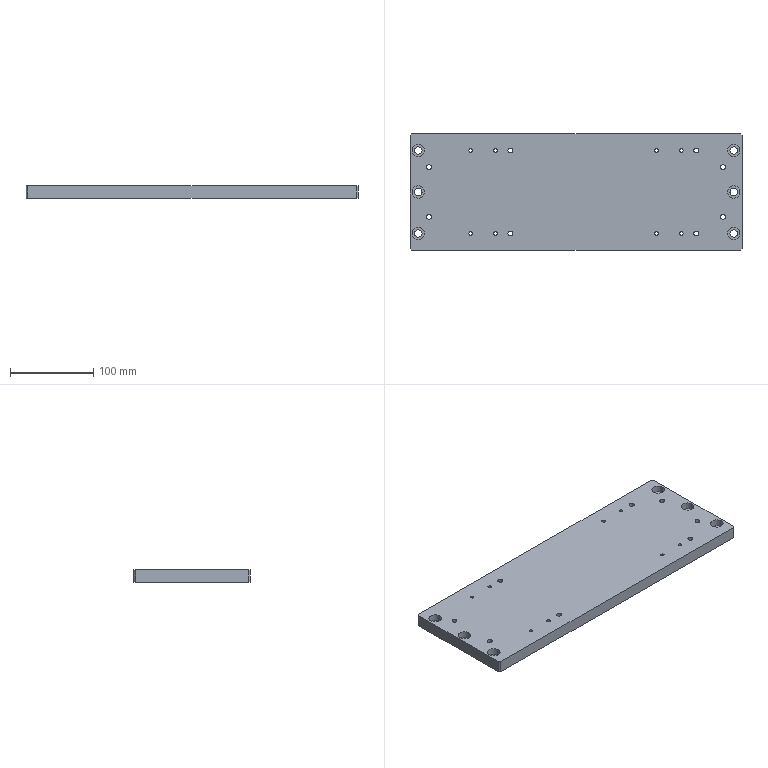Part | 1 solid | 52 faces | box 400 x 140 x 15 mm | volume 820295 mm3 | cylinder 32 | plane 16 | cone 4 | commonest cylinder face diameters 4.2 x8 6 x8 9 x6 15 x6 6.8 x4
STEP:
#1=CARTESIAN_POINT('',(-198.,70.,7.5));
#2=VERTEX_POINT('',#1);
#3=CARTESIAN_POINT('',(-200.,68.,7.5));
#4=VERTEX_POINT('',#3);
#5=CARTESIAN_POINT('',(-134.,134.,7.5));
#6=DIRECTION('',(-0.7071,-0.7071,0.));
#7=VECTOR('',#6,1000.);
#8=LINE('',#5,#7);
#9=EDGE_CURVE('',#2,#4,#8,.T.);
#10=ORIENTED_EDGE('',*,*,#9,.F.);
#11=CARTESIAN_POINT('',(-198.,70.,-7.5));
#12=VERTEX_POINT('',#11);
#13=CARTESIAN_POINT('',(-198.,70.,7.5));
#14=DIRECTION('',(0.,0.,1.));
#15=VECTOR('',#14,1000.);
#16=LINE('',#13,#15);
#17=EDGE_CURVE('',#12,#2,#16,.T.);
#18=ORIENTED_EDGE('',*,*,#17,.F.);
#19=CARTESIAN_POINT('',(-200.,68.,-7.5));
#20=VERTEX_POINT('',#19);
#21=CARTESIAN_POINT('',(-200.,68.,-7.5));
#22=DIRECTION('',(0.7071,0.7071,0.));
#23=VECTOR('',#22,1000.);
#24=LINE('',#21,#23);
#25=EDGE_CURVE('',#20,#12,#24,.T.);
#26=ORIENTED_EDGE('',*,*,#25,.F.);
#27=CARTESIAN_POINT('',(-200.,68.,7.5));
#28=DIRECTION('',(0.,0.,-1.));
#29=VECTOR('',#28,1000.);
#30=LINE('',#27,#29);
#31=EDGE_CURVE('',#4,#20,#30,.T.);
#32=ORIENTED_EDGE('',*,*,#31,.F.);
#33=EDGE_LOOP('',(#10,#18,#26,#32));
#34=FACE_BOUND('',#33,.T.);
#35=CARTESIAN_POINT('',(-200.,68.,7.5));
#36=DIRECTION('',(0.7071,-0.7071,0.));
#37=DIRECTION('',(0.,0.,-1.));
#38=AXIS2_PLACEMENT_3D('',#35,#36,#37);
#39=PLANE('',#38);
#40=ADVANCED_FACE('',(#34),#39,.F.);
#41=CARTESIAN_POINT('',(200.,68.,7.5));
#42=VERTEX_POINT('',#41);
#43=CARTESIAN_POINT('',(198.,70.,7.5));
#44=VERTEX_POINT('',#43);
#45=CARTESIAN_POINT('',(134.,134.,7.5));
#46=DIRECTION('',(-0.7071,0.7071,0.));
#47=VECTOR('',#46,1000.);
#48=LINE('',#45,#47);
#49=EDGE_CURVE('',#42,#44,#48,.T.);
#50=ORIENTED_EDGE('',*,*,#49,.F.);
#51=CARTESIAN_POINT('',(200.,68.,-7.5));
#52=VERTEX_POINT('',#51);
#53=CARTESIAN_POINT('',(200.,68.,7.5));
#54=DIRECTION('',(0.,0.,1.));
#55=VECTOR('',#54,1000.);
#56=LINE('',#53,#55);
#57=EDGE_CURVE('',#52,#42,#56,.T.);
#58=ORIENTED_EDGE('',*,*,#57,.F.);
#59=CARTESIAN_POINT('',(198.,70.,-7.5));
#60=VERTEX_POINT('',#59);
#61=CARTESIAN_POINT('',(198.,70.,-7.5));
#62=DIRECTION('',(0.7071,-0.7071,0.));
#63=VECTOR('',#62,1000.);
#64=LINE('',#61,#63);
#65=EDGE_CURVE('',#60,#52,#64,.T.);
#66=ORIENTED_EDGE('',*,*,#65,.F.);
#67=CARTESIAN_POINT('',(198.,70.,7.5));
#68=DIRECTION('',(0.,0.,-1.));
#69=VECTOR('',#68,1000.);
#70=LINE('',#67,#69);
#71=EDGE_CURVE('',#44,#60,#70,.T.);
#72=ORIENTED_EDGE('',*,*,#71,.F.);
#73=EDGE_LOOP('',(#50,#58,#66,#72));
#74=FACE_BOUND('',#73,.T.);
#75=CARTESIAN_POINT('',(198.,70.,7.5));
#76=DIRECTION('',(-0.7071,-0.7071,0.));
#77=DIRECTION('',(0.,0.,-1.));
#78=AXIS2_PLACEMENT_3D('',#75,#76,#77);
#79=PLANE('',#78);
#80=ADVANCED_FACE('',(#74),#79,.F.);
#81=CARTESIAN_POINT('',(-200.,-68.,7.5));
#82=VERTEX_POINT('',#81);
#83=CARTESIAN_POINT('',(-198.,-70.,7.5));
#84=VERTEX_POINT('',#83);
#85=CARTESIAN_POINT('',(-134.,-134.,7.5));
#86=DIRECTION('',(0.7071,-0.7071,0.));
#87=VECTOR('',#86,1000.);
#88=LINE('',#85,#87);
#89=EDGE_CURVE('',#82,#84,#88,.T.);
#90=ORIENTED_EDGE('',*,*,#89,.F.);
#91=CARTESIAN_POINT('',(-200.,-68.,-7.5));
#92=VERTEX_POINT('',#91);
#93=CARTESIAN_POINT('',(-200.,-68.,7.5));
#94=DIRECTION('',(0.,0.,1.));
#95=VECTOR('',#94,1000.);
#96=LINE('',#93,#95);
#97=EDGE_CURVE('',#92,#82,#96,.T.);
#98=ORIENTED_EDGE('',*,*,#97,.F.);
#99=CARTESIAN_POINT('',(-198.,-70.,-7.5));
#100=VERTEX_POINT('',#99);
#101=CARTESIAN_POINT('',(-198.,-70.,-7.5));
#102=DIRECTION('',(-0.7071,0.7071,0.));
#103=VECTOR('',#102,1000.);
#104=LINE('',#101,#103);
#105=EDGE_CURVE('',#100,#92,#104,.T.);
#106=ORIENTED_EDGE('',*,*,#105,.F.);
#107=CARTESIAN_POINT('',(-198.,-70.,7.5));
#108=DIRECTION('',(0.,0.,-1.));
#109=VECTOR('',#108,1000.);
#110=LINE('',#107,#109);
#111=EDGE_CURVE('',#84,#100,#110,.T.);
#112=ORIENTED_EDGE('',*,*,#111,.F.);
#113=EDGE_LOOP('',(#90,#98,#106,#112));
#114=FACE_BOUND('',#113,.T.);
#115=CARTESIAN_POINT('',(-198.,-70.,7.5));
#116=DIRECTION('',(0.7071,0.7071,0.));
#117=DIRECTION('',(0.,0.,-1.));
#118=AXIS2_PLACEMENT_3D('',#115,#116,#117);
#119=PLANE('',#118);
#120=ADVANCED_FACE('',(#114),#119,.F.);
#121=CARTESIAN_POINT('',(198.,-70.,7.5));
#122=VERTEX_POINT('',#121);
#123=CARTESIAN_POINT('',(200.,-68.,7.5));
#124=VERTEX_POINT('',#123);
#125=CARTESIAN_POINT('',(134.,-134.,7.5));
#126=DIRECTION('',(0.7071,0.7071,0.));
#127=VECTOR('',#126,1000.);
#128=LINE('',#125,#127);
#129=EDGE_CURVE('',#122,#124,#128,.T.);
#130=ORIENTED_EDGE('',*,*,#129,.F.);
#131=CARTESIAN_POINT('',(198.,-70.,-7.5));
#132=VERTEX_POINT('',#131);
#133=CARTESIAN_POINT('',(198.,-70.,7.5));
#134=DIRECTION('',(0.,0.,1.));
#135=VECTOR('',#134,1000.);
#136=LINE('',#133,#135);
#137=EDGE_CURVE('',#132,#122,#136,.T.);
#138=ORIENTED_EDGE('',*,*,#137,.F.);
#139=CARTESIAN_POINT('',(200.,-68.,-7.5));
#140=VERTEX_POINT('',#139);
#141=CARTESIAN_POINT('',(200.,-68.,-7.5));
#142=DIRECTION('',(-0.7071,-0.7071,0.));
#143=VECTOR('',#142,1000.);
#144=LINE('',#141,#143);
#145=EDGE_CURVE('',#140,#132,#144,.T.);
#146=ORIENTED_EDGE('',*,*,#145,.F.);
#147=CARTESIAN_POINT('',(200.,-68.,7.5));
#148=DIRECTION('',(0.,0.,-1.));
#149=VECTOR('',#148,1000.);
#150=LINE('',#147,#149);
#151=EDGE_CURVE('',#124,#140,#150,.T.);
#152=ORIENTED_EDGE('',*,*,#151,.F.);
#153=EDGE_LOOP('',(#130,#138,#146,#152));
#154=FACE_BOUND('',#153,.T.);
#155=CARTESIAN_POINT('',(200.,-68.,7.5));
#156=DIRECTION('',(-0.7071,0.7071,0.));
#157=DIRECTION('',(0.,0.,-1.));
#158=AXIS2_PLACEMENT_3D('',#155,#156,#157);
#159=PLANE('',#158);
#160=ADVANCED_FACE('',(#154),#159,.F.);
#161=CARTESIAN_POINT('',(-182.5,50.,-1.1));
#162=VERTEX_POINT('',#161);
#163=CARTESIAN_POINT('',(-190.,50.,-1.1));
#164=DIRECTION('',(0.,0.,1.));
#165=DIRECTION('',(1.,0.,0.));
#166=AXIS2_PLACEMENT_3D('',#163,#164,#165);
#167=CIRCLE('',#166,7.5);
#168=EDGE_CURVE('',#162,#162,#167,.T.);
#169=ORIENTED_EDGE('',*,*,#168,.T.);
#170=EDGE_LOOP('',(#169));
#171=FACE_BOUND('',#170,.T.);
#172=CARTESIAN_POINT('',(-185.5,50.,-1.1));
#173=VERTEX_POINT('',#172);
#174=CARTESIAN_POINT('',(-190.,50.,-1.1));
#175=DIRECTION('',(0.,0.,1.));
#176=DIRECTION('',(1.,0.,0.));
#177=AXIS2_PLACEMENT_3D('',#174,#175,#176);
#178=CIRCLE('',#177,4.5);
#179=EDGE_CURVE('',#173,#173,#178,.T.);
#180=ORIENTED_EDGE('',*,*,#179,.F.);
#181=EDGE_LOOP('',(#180));
#182=FACE_BOUND('',#181,.T.);
#183=CARTESIAN_POINT('',(-185.5,50.,-1.1));
#184=DIRECTION('',(0.,0.,-1.));
#185=DIRECTION('',(-1.,0.,0.));
#186=AXIS2_PLACEMENT_3D('',#183,#184,#185);
#187=PLANE('',#186);
#188=ADVANCED_FACE('',(#171,#182),#187,.F.);
#189=CARTESIAN_POINT('',(182.5,50.,-1.1));
#190=VERTEX_POINT('',#189);
#191=CARTESIAN_POINT('',(190.,50.,-1.1));
#192=DIRECTION('',(0.,0.,1.));
#193=DIRECTION('',(-1.,0.,0.));
#194=AXIS2_PLACEMENT_3D('',#191,#192,#193);
#195=CIRCLE('',#194,7.5);
#196=EDGE_CURVE('',#190,#190,#195,.T.);
#197=ORIENTED_EDGE('',*,*,#196,.T.);
#198=EDGE_LOOP('',(#197));
#199=FACE_BOUND('',#198,.T.);
#200=CARTESIAN_POINT('',(185.5,50.,-1.1));
#201=VERTEX_POINT('',#200);
#202=CARTESIAN_POINT('',(190.,50.,-1.1));
#203=DIRECTION('',(0.,0.,1.));
#204=DIRECTION('',(-1.,0.,0.));
#205=AXIS2_PLACEMENT_3D('',#202,#203,#204);
#206=CIRCLE('',#205,4.5);
#207=EDGE_CURVE('',#201,#201,#206,.T.);
#208=ORIENTED_EDGE('',*,*,#207,.F.);
#209=EDGE_LOOP('',(#208));
#210=FACE_BOUND('',#209,.T.);
#211=CARTESIAN_POINT('',(-185.5,50.,-1.1));
#212=DIRECTION('',(0.,0.,-1.));
#213=DIRECTION('',(-1.,0.,0.));
#214=AXIS2_PLACEMENT_3D('',#211,#212,#213);
#215=PLANE('',#214);
#216=ADVANCED_FACE('',(#199,#210),#215,.F.);
#217=CARTESIAN_POINT('',(-197.5,-50.,-1.1));
#218=VERTEX_POINT('',#217);
#219=CARTESIAN_POINT('',(-190.,-50.,-1.1));
#220=DIRECTION('',(0.,0.,1.));
#221=DIRECTION('',(-1.,0.,0.));
#222=AXIS2_PLACEMENT_3D('',#219,#220,#221);
#223=CIRCLE('',#222,7.5);
#224=EDGE_CURVE('',#218,#218,#223,.T.);
#225=ORIENTED_EDGE('',*,*,#224,.T.);
#226=EDGE_LOOP('',(#225));
#227=FACE_BOUND('',#226,.T.);
#228=CARTESIAN_POINT('',(-194.5,-50.,-1.1));
#229=VERTEX_POINT('',#228);
#230=CARTESIAN_POINT('',(-190.,-50.,-1.1));
#231=DIRECTION('',(0.,0.,1.));
#232=DIRECTION('',(-1.,0.,0.));
#233=AXIS2_PLACEMENT_3D('',#230,#231,#232);
#234=CIRCLE('',#233,4.5);
#235=EDGE_CURVE('',#229,#229,#234,.T.);
#236=ORIENTED_EDGE('',*,*,#235,.F.);
#237=EDGE_LOOP('',(#236));
#238=FACE_BOUND('',#237,.T.);
#239=CARTESIAN_POINT('',(-185.5,50.,-1.1));
#240=DIRECTION('',(0.,0.,-1.));
#241=DIRECTION('',(-1.,0.,0.));
#242=AXIS2_PLACEMENT_3D('',#239,#240,#241);
#243=PLANE('',#242);
#244=ADVANCED_FACE('',(#227,#238),#243,.F.);
#245=CARTESIAN_POINT('',(182.5,-50.,-1.1));
#246=VERTEX_POINT('',#245);
#247=CARTESIAN_POINT('',(190.,-50.,-1.1));
#248=DIRECTION('',(0.,0.,1.));
#249=DIRECTION('',(-1.,0.,0.));
#250=AXIS2_PLACEMENT_3D('',#247,#248,#249);
#251=CIRCLE('',#250,7.5);
#252=EDGE_CURVE('',#246,#246,#251,.T.);
#253=ORIENTED_EDGE('',*,*,#252,.T.);
#254=EDGE_LOOP('',(#253));
#255=FACE_BOUND('',#254,.T.);
#256=CARTESIAN_POINT('',(185.5,-50.,-1.1));
#257=VERTEX_POINT('',#256);
#258=CARTESIAN_POINT('',(190.,-50.,-1.1));
#259=DIRECTION('',(0.,0.,1.));
#260=DIRECTION('',(-1.,0.,0.));
#261=AXIS2_PLACEMENT_3D('',#258,#259,#260);
#262=CIRCLE('',#261,4.5);
#263=EDGE_CURVE('',#257,#257,#262,.T.);
#264=ORIENTED_EDGE('',*,*,#263,.F.);
#265=EDGE_LOOP('',(#264));
#266=FACE_BOUND('',#265,.T.);
#267=CARTESIAN_POINT('',(-185.5,50.,-1.1));
#268=DIRECTION('',(0.,0.,-1.));
#269=DIRECTION('',(-1.,0.,0.));
#270=AXIS2_PLACEMENT_3D('',#267,#268,#269);
#271=PLANE('',#270);
#272=ADVANCED_FACE('',(#255,#266),#271,.F.);
#273=CARTESIAN_POINT('',(182.5,0.,-1.1));
#274=VERTEX_POINT('',#273);
#275=CARTESIAN_POINT('',(190.,0.,-1.1));
#276=DIRECTION('',(0.,0.,1.));
#277=DIRECTION('',(-1.,0.,0.));
#278=AXIS2_PLACEMENT_3D('',#275,#276,#277);
#279=CIRCLE('',#278,7.5);
#280=EDGE_CURVE('',#274,#274,#279,.T.);
#281=ORIENTED_EDGE('',*,*,#280,.T.);
#282=EDGE_LOOP('',(#281));
#283=FACE_BOUND('',#282,.T.);
#284=CARTESIAN_POINT('',(185.5,0.,-1.1));
#285=VERTEX_POINT('',#284);
#286=CARTESIAN_POINT('',(190.,0.,-1.1));
#287=DIRECTION('',(0.,0.,1.));
#288=DIRECTION('',(-1.,0.,0.));
#289=AXIS2_PLACEMENT_3D('',#286,#287,#288);
#290=CIRCLE('',#289,4.5);
#291=EDGE_CURVE('',#285,#285,#290,.T.);
#292=ORIENTED_EDGE('',*,*,#291,.F.);
#293=EDGE_LOOP('',(#292));
#294=FACE_BOUND('',#293,.T.);
#295=CARTESIAN_POINT('',(-185.5,50.,-1.1));
#296=DIRECTION('',(0.,0.,-1.));
#297=DIRECTION('',(-1.,0.,0.));
#298=AXIS2_PLACEMENT_3D('',#295,#296,#297);
#299=PLANE('',#298);
#300=ADVANCED_FACE('',(#283,#294),#299,.F.);
#301=CARTESIAN_POINT('',(-197.5,0.,-1.1));
#302=VERTEX_POINT('',#301);
#303=CARTESIAN_POINT('',(-190.,0.,-1.1));
#304=DIRECTION('',(0.,0.,1.));
#305=DIRECTION('',(-1.,0.,0.));
#306=AXIS2_PLACEMENT_3D('',#303,#304,#305);
#307=CIRCLE('',#306,7.5);
#308=EDGE_CURVE('',#302,#302,#307,.T.);
#309=ORIENTED_EDGE('',*,*,#308,.T.);
#310=EDGE_LOOP('',(#309));
#311=FACE_BOUND('',#310,.T.);
#312=CARTESIAN_POINT('',(-194.5,0.,-1.1));
#313=VERTEX_POINT('',#312);
#314=CARTESIAN_POINT('',(-190.,0.,-1.1));
#315=DIRECTION('',(0.,0.,1.));
#316=DIRECTION('',(-1.,0.,0.));
#317=AXIS2_PLACEMENT_3D('',#314,#315,#316);
#318=CIRCLE('',#317,4.5);
#319=EDGE_CURVE('',#313,#313,#318,.T.);
#320=ORIENTED_EDGE('',*,*,#319,.F.);
#321=EDGE_LOOP('',(#320));
#322=FACE_BOUND('',#321,.T.);
#323=CARTESIAN_POINT('',(-185.5,50.,-1.1));
#324=DIRECTION('',(0.,0.,-1.));
#325=DIRECTION('',(-1.,0.,0.));
#326=AXIS2_PLACEMENT_3D('',#323,#324,#325);
#327=PLANE('',#326);
#328=ADVANCED_FACE('',(#311,#322),#327,.F.);
#329=CARTESIAN_POINT('',(200.,-70.,-7.5));
#330=DIRECTION('',(0.,1.,0.));
#331=VECTOR('',#330,1000.);
#332=LINE('',#329,#331);
#333=EDGE_CURVE('',#140,#52,#332,.T.);
#334=ORIENTED_EDGE('',*,*,#333,.F.);
#335=ORIENTED_EDGE('',*,*,#145,.T.);
#336=CARTESIAN_POINT('',(200.,-70.,-7.5));
#337=DIRECTION('',(1.,0.,0.));
#338=VECTOR('',#337,1000.);
#339=LINE('',#336,#338);
#340=EDGE_CURVE('',#100,#132,#339,.T.);
#341=ORIENTED_EDGE('',*,*,#340,.F.);
#342=ORIENTED_EDGE('',*,*,#105,.T.);
#343=CARTESIAN_POINT('',(-200.,-70.,-7.5));
#344=DIRECTION('',(0.,-1.,0.));
#345=VECTOR('',#344,1000.);
#346=LINE('',#343,#345);
#347=EDGE_CURVE('',#20,#92,#346,.T.);
#348=ORIENTED_EDGE('',*,*,#347,.F.);
#349=ORIENTED_EDGE('',*,*,#25,.T.);
#350=CARTESIAN_POINT('',(200.,70.,-7.5));
#351=DIRECTION('',(-1.,0.,0.));
#352=VECTOR('',#351,1000.);
#353=LINE('',#350,#352);
#354=EDGE_CURVE('',#60,#12,#353,.T.);
#355=ORIENTED_EDGE('',*,*,#354,.F.);
#356=ORIENTED_EDGE('',*,*,#65,.T.);
#357=EDGE_LOOP('',(#334,#335,#341,#342,#348,#349,#355,#356));
#358=FACE_BOUND('',#357,.T.);
#359=CARTESIAN_POINT('',(-124.9,-50.,-7.5));
#360=VERTEX_POINT('',#359);
#361=CARTESIAN_POINT('',(-127.,-50.,-7.5));
#362=DIRECTION('',(0.,0.,1.));
#363=DIRECTION('',(1.,0.,0.));
#364=AXIS2_PLACEMENT_3D('',#361,#362,#363);
#365=CIRCLE('',#364,2.1);
#366=EDGE_CURVE('',#360,#360,#365,.T.);
#367=ORIENTED_EDGE('',*,*,#366,.T.);
#368=EDGE_LOOP('',(#367));
#369=FACE_BOUND('',#368,.T.);
#370=CARTESIAN_POINT('',(-94.9,-50.,-7.5));
#371=VERTEX_POINT('',#370);
#372=CARTESIAN_POINT('',(-97.,-50.,-7.5));
#373=DIRECTION('',(0.,0.,1.));
#374=DIRECTION('',(1.,0.,0.));
#375=AXIS2_PLACEMENT_3D('',#372,#373,#374);
#376=CIRCLE('',#375,2.1);
#377=EDGE_CURVE('',#371,#371,#376,.T.);
#378=ORIENTED_EDGE('',*,*,#377,.T.);
#379=EDGE_LOOP('',(#378));
#380=FACE_BOUND('',#379,.T.);
#381=CARTESIAN_POINT('',(-94.9,50.,-7.5));
#382=VERTEX_POINT('',#381);
#383=CARTESIAN_POINT('',(-97.,50.,-7.5));
#384=DIRECTION('',(0.,0.,1.));
#385=DIRECTION('',(1.,0.,0.));
#386=AXIS2_PLACEMENT_3D('',#383,#384,#385);
#387=CIRCLE('',#386,2.1);
#388=EDGE_CURVE('',#382,#382,#387,.T.);
#389=ORIENTED_EDGE('',*,*,#388,.T.);
#390=EDGE_LOOP('',(#389));
#391=FACE_BOUND('',#390,.T.);
#392=CARTESIAN_POINT('',(-124.9,50.,-7.5));
#393=VERTEX_POINT('',#392);
#394=CARTESIAN_POINT('',(-127.,50.,-7.5));
#395=DIRECTION('',(0.,0.,1.));
#396=DIRECTION('',(1.,0.,0.));
#397=AXIS2_PLACEMENT_3D('',#394,#395,#396);
#398=CIRCLE('',#397,2.1);
#399=EDGE_CURVE('',#393,#393,#398,.T.);
#400=ORIENTED_EDGE('',*,*,#399,.T.);
#401=EDGE_LOOP('',(#400));
#402=FACE_BOUND('',#401,.T.);
#403=CARTESIAN_POINT('',(-76.,-50.,-7.5));
#404=VERTEX_POINT('',#403);
#405=CARTESIAN_POINT('',(-79.,-50.,-7.5));
#406=DIRECTION('',(0.,0.,1.));
#407=DIRECTION('',(1.,0.,0.));
#408=AXIS2_PLACEMENT_3D('',#405,#406,#407);
#409=CIRCLE('',#408,3.);
#410=EDGE_CURVE('',#404,#404,#409,.T.);
#411=ORIENTED_EDGE('',*,*,#410,.T.);
#412=EDGE_LOOP('',(#411));
#413=FACE_BOUND('',#412,.T.);
#414=CARTESIAN_POINT('',(-76.,50.,-7.5));
#415=VERTEX_POINT('',#414);
#416=CARTESIAN_POINT('',(-79.,50.,-7.5));
#417=DIRECTION('',(0.,0.,1.));
#418=DIRECTION('',(1.,0.,0.));
#419=AXIS2_PLACEMENT_3D('',#416,#417,#418);
#420=CIRCLE('',#419,3.);
#421=EDGE_CURVE('',#415,#415,#420,.T.);
#422=ORIENTED_EDGE('',*,*,#421,.T.);
#423=EDGE_LOOP('',(#422));
#424=FACE_BOUND('',#423,.T.);
#425=CARTESIAN_POINT('',(99.1,50.,-7.5));
#426=VERTEX_POINT('',#425);
#427=CARTESIAN_POINT('',(97.,50.,-7.5));
#428=DIRECTION('',(0.,0.,1.));
#429=DIRECTION('',(1.,0.,0.));
#430=AXIS2_PLACEMENT_3D('',#427,#428,#429);
#431=CIRCLE('',#430,2.1);
#432=EDGE_CURVE('',#426,#426,#431,.T.);
#433=ORIENTED_EDGE('',*,*,#432,.T.);
#434=EDGE_LOOP('',(#433));
#435=FACE_BOUND('',#434,.T.);
#436=CARTESIAN_POINT('',(99.1,-50.,-7.5));
#437=VERTEX_POINT('',#436);
#438=CARTESIAN_POINT('',(97.,-50.,-7.5));
#439=DIRECTION('',(0.,0.,1.));
#440=DIRECTION('',(1.,0.,0.));
#441=AXIS2_PLACEMENT_3D('',#438,#439,#440);
#442=CIRCLE('',#441,2.1);
#443=EDGE_CURVE('',#437,#437,#442,.T.);
#444=ORIENTED_EDGE('',*,*,#443,.T.);
#445=EDGE_LOOP('',(#444));
#446=FACE_BOUND('',#445,.T.);
#447=CARTESIAN_POINT('',(129.1,-50.,-7.5));
#448=VERTEX_POINT('',#447);
#449=CARTESIAN_POINT('',(127.,-50.,-7.5));
#450=DIRECTION('',(0.,0.,1.));
#451=DIRECTION('',(1.,0.,0.));
#452=AXIS2_PLACEMENT_3D('',#449,#450,#451);
#453=CIRCLE('',#452,2.1);
#454=EDGE_CURVE('',#448,#448,#453,.T.);
#455=ORIENTED_EDGE('',*,*,#454,.T.);
#456=EDGE_LOOP('',(#455));
#457=FACE_BOUND('',#456,.T.);
#458=CARTESIAN_POINT('',(129.1,50.,-7.5));
#459=VERTEX_POINT('',#458);
#460=CARTESIAN_POINT('',(127.,50.,-7.5));
#461=DIRECTION('',(0.,0.,1.));
#462=DIRECTION('',(1.,0.,0.));
#463=AXIS2_PLACEMENT_3D('',#460,#461,#462);
#464=CIRCLE('',#463,2.1);
#465=EDGE_CURVE('',#459,#459,#464,.T.);
#466=ORIENTED_EDGE('',*,*,#465,.T.);
#467=EDGE_LOOP('',(#466));
#468=FACE_BOUND('',#467,.T.);
#469=CARTESIAN_POINT('',(148.,-50.,-7.5));
#470=VERTEX_POINT('',#469);
#471=CARTESIAN_POINT('',(145.,-50.,-7.5));
#472=DIRECTION('',(0.,0.,1.));
#473=DIRECTION('',(1.,0.,0.));
#474=AXIS2_PLACEMENT_3D('',#471,#472,#473);
#475=CIRCLE('',#474,3.);
#476=EDGE_CURVE('',#470,#470,#475,.T.);
#477=ORIENTED_EDGE('',*,*,#476,.T.);
#478=EDGE_LOOP('',(#477));
#479=FACE_BOUND('',#478,.T.);
#480=CARTESIAN_POINT('',(148.,50.,-7.5));
#481=VERTEX_POINT('',#480);
#482=CARTESIAN_POINT('',(145.,50.,-7.5));
#483=DIRECTION('',(0.,0.,1.));
#484=DIRECTION('',(1.,0.,0.));
#485=AXIS2_PLACEMENT_3D('',#482,#483,#484);
#486=CIRCLE('',#485,3.);
#487=EDGE_CURVE('',#481,#481,#486,.T.);
#488=ORIENTED_EDGE('',*,*,#487,.T.);
#489=EDGE_LOOP('',(#488));
#490=FACE_BOUND('',#489,.T.);
#491=CARTESIAN_POINT('',(-185.5,0.,-7.5));
#492=VERTEX_POINT('',#491);
#493=CARTESIAN_POINT('',(-190.,0.,-7.5));
#494=DIRECTION('',(0.,0.,1.));
#495=DIRECTION('',(1.,0.,0.));
#496=AXIS2_PLACEMENT_3D('',#493,#494,#495);
#497=CIRCLE('',#496,4.5);
#498=EDGE_CURVE('',#492,#492,#497,.T.);
#499=ORIENTED_EDGE('',*,*,#498,.T.);
#500=EDGE_LOOP('',(#499));
#501=FACE_BOUND('',#500,.T.);
#502=CARTESIAN_POINT('',(194.5,0.,-7.5));
#503=VERTEX_POINT('',#502);
#504=CARTESIAN_POINT('',(190.,0.,-7.5));
#505=DIRECTION('',(0.,0.,1.));
#506=DIRECTION('',(1.,0.,0.));
#507=AXIS2_PLACEMENT_3D('',#504,#505,#506);
#508=CIRCLE('',#507,4.5);
#509=EDGE_CURVE('',#503,#503,#508,.T.);
#510=ORIENTED_EDGE('',*,*,#509,.T.);
#511=EDGE_LOOP('',(#510));
#512=FACE_BOUND('',#511,.T.);
#513=CARTESIAN_POINT('',(194.5,-50.,-7.5));
#514=VERTEX_POINT('',#513);
#515=CARTESIAN_POINT('',(190.,-50.,-7.5));
#516=DIRECTION('',(0.,0.,1.));
#517=DIRECTION('',(1.,0.,0.));
#518=AXIS2_PLACEMENT_3D('',#515,#516,#517);
#519=CIRCLE('',#518,4.5);
#520=EDGE_CURVE('',#514,#514,#519,.T.);
#521=ORIENTED_EDGE('',*,*,#520,.T.);
#522=EDGE_LOOP('',(#521));
#523=FACE_BOUND('',#522,.T.);
#524=CARTESIAN_POINT('',(-185.5,-50.,-7.5));
#525=VERTEX_POINT('',#524);
#526=CARTESIAN_POINT('',(-190.,-50.,-7.5));
#527=DIRECTION('',(0.,0.,1.));
#528=DIRECTION('',(1.,0.,0.));
#529=AXIS2_PLACEMENT_3D('',#526,#527,#528);
#530=CIRCLE('',#529,4.5);
#531=EDGE_CURVE('',#525,#525,#530,.T.);
#532=ORIENTED_EDGE('',*,*,#531,.T.);
#533=EDGE_LOOP('',(#532));
#534=FACE_BOUND('',#533,.T.);
#535=CARTESIAN_POINT('',(194.5,50.,-7.5));
#536=VERTEX_POINT('',#535);
#537=CARTESIAN_POINT('',(190.,50.,-7.5));
#538=DIRECTION('',(0.,0.,1.));
#539=DIRECTION('',(1.,0.,0.));
#540=AXIS2_PLACEMENT_3D('',#537,#538,#539);
#541=CIRCLE('',#540,4.5);
#542=EDGE_CURVE('',#536,#536,#541,.T.);
#543=ORIENTED_EDGE('',*,*,#542,.T.);
#544=EDGE_LOOP('',(#543));
#545=FACE_BOUND('',#544,.T.);
#546=CARTESIAN_POINT('',(-185.5,50.,-7.5));
#547=VERTEX_POINT('',#546);
#548=CARTESIAN_POINT('',(-190.,50.,-7.5));
#549=DIRECTION('',(0.,0.,1.));
#550=DIRECTION('',(1.,0.,0.));
#551=AXIS2_PLACEMENT_3D('',#548,#549,#550);
#552=CIRCLE('',#551,4.5);
#553=EDGE_CURVE('',#547,#547,#552,.T.);
#554=ORIENTED_EDGE('',*,*,#553,.T.);
#555=EDGE_LOOP('',(#554));
#556=FACE_BOUND('',#555,.T.);
#557=CARTESIAN_POINT('',(-174.,-30.,-7.5));
#558=VERTEX_POINT('',#557);
#559=CARTESIAN_POINT('',(-177.,-30.,-7.5));
#560=DIRECTION('',(0.,0.,1.));
#561=DIRECTION('',(1.,0.,0.));
#562=AXIS2_PLACEMENT_3D('',#559,#560,#561);
#563=CIRCLE('',#562,3.);
#564=EDGE_CURVE('',#558,#558,#563,.T.);
#565=ORIENTED_EDGE('',*,*,#564,.T.);
#566=EDGE_LOOP('',(#565));
#567=FACE_BOUND('',#566,.T.);
#568=CARTESIAN_POINT('',(-174.,30.,-7.5));
#569=VERTEX_POINT('',#568);
#570=CARTESIAN_POINT('',(-177.,30.,-7.5));
#571=DIRECTION('',(0.,0.,1.));
#572=DIRECTION('',(1.,0.,0.));
#573=AXIS2_PLACEMENT_3D('',#570,#571,#572);
#574=CIRCLE('',#573,3.);
#575=EDGE_CURVE('',#569,#569,#574,.T.);
#576=ORIENTED_EDGE('',*,*,#575,.T.);
#577=EDGE_LOOP('',(#576));
#578=FACE_BOUND('',#577,.T.);
#579=CARTESIAN_POINT('',(180.,-30.,-7.5));
#580=VERTEX_POINT('',#579);
#581=CARTESIAN_POINT('',(177.,-30.,-7.5));
#582=DIRECTION('',(0.,0.,1.));
#583=DIRECTION('',(1.,0.,0.));
#584=AXIS2_PLACEMENT_3D('',#581,#582,#583);
#585=CIRCLE('',#584,3.);
#586=EDGE_CURVE('',#580,#580,#585,.T.);
#587=ORIENTED_EDGE('',*,*,#586,.T.);
#588=EDGE_LOOP('',(#587));
#589=FACE_BOUND('',#588,.T.);
#590=CARTESIAN_POINT('',(180.,30.,-7.5));
#591=VERTEX_POINT('',#590);
#592=CARTESIAN_POINT('',(177.,30.,-7.5));
#593=DIRECTION('',(0.,0.,1.));
#594=DIRECTION('',(1.,0.,0.));
#595=AXIS2_PLACEMENT_3D('',#592,#593,#594);
#596=CIRCLE('',#595,3.);
#597=EDGE_CURVE('',#591,#591,#596,.T.);
#598=ORIENTED_EDGE('',*,*,#597,.T.);
#599=EDGE_LOOP('',(#598));
#600=FACE_BOUND('',#599,.T.);
#601=CARTESIAN_POINT('',(0.,0.,-7.5));
#602=DIRECTION('',(0.,0.,1.));
#603=DIRECTION('',(1.,0.,0.));
#604=AXIS2_PLACEMENT_3D('',#601,#602,#603);
#605=PLANE('',#604);
#606=ADVANCED_FACE('',(#358,#369,#380,#391,#402,#413,#424,#435,#446,#457,#468,#479,#490,#501,#512,#523,#534,#545,#556,#567,#578,#589,#600),#605,.F.);
#607=CARTESIAN_POINT('',(200.,-70.,7.5));
#608=DIRECTION('',(1.,0.,0.));
#609=VECTOR('',#608,1000.);
#610=LINE('',#607,#609);
#611=EDGE_CURVE('',#84,#122,#610,.T.);
#612=ORIENTED_EDGE('',*,*,#611,.T.);
#613=ORIENTED_EDGE('',*,*,#129,.T.);
#614=CARTESIAN_POINT('',(200.,-70.,7.5));
#615=DIRECTION('',(0.,1.,0.));
#616=VECTOR('',#615,1000.);
#617=LINE('',#614,#616);
#618=EDGE_CURVE('',#124,#42,#617,.T.);
#619=ORIENTED_EDGE('',*,*,#618,.T.);
#620=ORIENTED_EDGE('',*,*,#49,.T.);
#621=CARTESIAN_POINT('',(200.,70.,7.5));
#622=DIRECTION('',(-1.,0.,0.));
#623=VECTOR('',#622,1000.);
#624=LINE('',#621,#623);
#625=EDGE_CURVE('',#44,#2,#624,.T.);
#626=ORIENTED_EDGE('',*,*,#625,.T.);
#627=ORIENTED_EDGE('',*,*,#9,.T.);
#628=CARTESIAN_POINT('',(-200.,-70.,7.5));
#629=DIRECTION('',(0.,-1.,0.));
#630=VECTOR('',#629,1000.);
#631=LINE('',#628,#630);
#632=EDGE_CURVE('',#4,#82,#631,.T.);
#633=ORIENTED_EDGE('',*,*,#632,.T.);
#634=ORIENTED_EDGE('',*,*,#89,.T.);
#635=EDGE_LOOP('',(#612,#613,#619,#620,#626,#627,#633,#634));
#636=FACE_BOUND('',#635,.T.);
#637=CARTESIAN_POINT('',(-124.9,-50.,7.5));
#638=VERTEX_POINT('',#637);
#639=CARTESIAN_POINT('',(-127.,-50.,7.5));
#640=DIRECTION('',(0.,0.,1.));
#641=DIRECTION('',(1.,0.,0.));
#642=AXIS2_PLACEMENT_3D('',#639,#640,#641);
#643=CIRCLE('',#642,2.1);
#644=EDGE_CURVE('',#638,#638,#643,.T.);
#645=ORIENTED_EDGE('',*,*,#644,.F.);
#646=EDGE_LOOP('',(#645));
#647=FACE_BOUND('',#646,.T.);
#648=CARTESIAN_POINT('',(-94.9,-50.,7.5));
#649=VERTEX_POINT('',#648);
#650=CARTESIAN_POINT('',(-97.,-50.,7.5));
#651=DIRECTION('',(0.,0.,1.));
#652=DIRECTION('',(1.,0.,0.));
#653=AXIS2_PLACEMENT_3D('',#650,#651,#652);
#654=CIRCLE('',#653,2.1);
#655=EDGE_CURVE('',#649,#649,#654,.T.);
#656=ORIENTED_EDGE('',*,*,#655,.F.);
#657=EDGE_LOOP('',(#656));
#658=FACE_BOUND('',#657,.T.);
#659=CARTESIAN_POINT('',(-94.9,50.,7.5));
#660=VERTEX_POINT('',#659);
#661=CARTESIAN_POINT('',(-97.,50.,7.5));
#662=DIRECTION('',(0.,0.,1.));
#663=DIRECTION('',(1.,0.,0.));
#664=AXIS2_PLACEMENT_3D('',#661,#662,#663);
#665=CIRCLE('',#664,2.1);
#666=EDGE_CURVE('',#660,#660,#665,.T.);
#667=ORIENTED_EDGE('',*,*,#666,.F.);
#668=EDGE_LOOP('',(#667));
#669=FACE_BOUND('',#668,.T.);
#670=CARTESIAN_POINT('',(-124.9,50.,7.5));
#671=VERTEX_POINT('',#670);
#672=CARTESIAN_POINT('',(-127.,50.,7.5));
#673=DIRECTION('',(0.,0.,1.));
#674=DIRECTION('',(1.,0.,0.));
#675=AXIS2_PLACEMENT_3D('',#672,#673,#674);
#676=CIRCLE('',#675,2.1);
#677=EDGE_CURVE('',#671,#671,#676,.T.);
#678=ORIENTED_EDGE('',*,*,#677,.F.);
#679=EDGE_LOOP('',(#678));
#680=FACE_BOUND('',#679,.T.);
#681=CARTESIAN_POINT('',(-76.,-50.,7.5));
#682=VERTEX_POINT('',#681);
#683=CARTESIAN_POINT('',(-79.,-50.,7.5));
#684=DIRECTION('',(0.,0.,1.));
#685=DIRECTION('',(1.,0.,0.));
#686=AXIS2_PLACEMENT_3D('',#683,#684,#685);
#687=CIRCLE('',#686,3.);
#688=EDGE_CURVE('',#682,#682,#687,.T.);
#689=ORIENTED_EDGE('',*,*,#688,.F.);
#690=EDGE_LOOP('',(#689));
#691=FACE_BOUND('',#690,.T.);
#692=CARTESIAN_POINT('',(-76.,50.,7.5));
#693=VERTEX_POINT('',#692);
#694=CARTESIAN_POINT('',(-79.,50.,7.5));
#695=DIRECTION('',(0.,0.,1.));
#696=DIRECTION('',(1.,0.,0.));
#697=AXIS2_PLACEMENT_3D('',#694,#695,#696);
#698=CIRCLE('',#697,3.);
#699=EDGE_CURVE('',#693,#693,#698,.T.);
#700=ORIENTED_EDGE('',*,*,#699,.F.);
#701=EDGE_LOOP('',(#700));
#702=FACE_BOUND('',#701,.T.);
#703=CARTESIAN_POINT('',(99.1,50.,7.5));
#704=VERTEX_POINT('',#703);
#705=CARTESIAN_POINT('',(97.,50.,7.5));
#706=DIRECTION('',(0.,0.,1.));
#707=DIRECTION('',(1.,0.,0.));
#708=AXIS2_PLACEMENT_3D('',#705,#706,#707);
#709=CIRCLE('',#708,2.1);
#710=EDGE_CURVE('',#704,#704,#709,.T.);
#711=ORIENTED_EDGE('',*,*,#710,.F.);
#712=EDGE_LOOP('',(#711));
#713=FACE_BOUND('',#712,.T.);
#714=CARTESIAN_POINT('',(99.1,-50.,7.5));
#715=VERTEX_POINT('',#714);
#716=CARTESIAN_POINT('',(97.,-50.,7.5));
#717=DIRECTION('',(0.,0.,1.));
#718=DIRECTION('',(1.,0.,0.));
#719=AXIS2_PLACEMENT_3D('',#716,#717,#718);
#720=CIRCLE('',#719,2.1);
#721=EDGE_CURVE('',#715,#715,#720,.T.);
#722=ORIENTED_EDGE('',*,*,#721,.F.);
#723=EDGE_LOOP('',(#722));
#724=FACE_BOUND('',#723,.T.);
#725=CARTESIAN_POINT('',(129.1,-50.,7.5));
#726=VERTEX_POINT('',#725);
#727=CARTESIAN_POINT('',(127.,-50.,7.5));
#728=DIRECTION('',(0.,0.,1.));
#729=DIRECTION('',(1.,0.,0.));
#730=AXIS2_PLACEMENT_3D('',#727,#728,#729);
#731=CIRCLE('',#730,2.1);
#732=EDGE_CURVE('',#726,#726,#731,.T.);
#733=ORIENTED_EDGE('',*,*,#732,.F.);
#734=EDGE_LOOP('',(#733));
#735=FACE_BOUND('',#734,.T.);
#736=CARTESIAN_POINT('',(129.1,50.,7.5));
#737=VERTEX_POINT('',#736);
#738=CARTESIAN_POINT('',(127.,50.,7.5));
#739=DIRECTION('',(0.,0.,1.));
#740=DIRECTION('',(1.,0.,0.));
#741=AXIS2_PLACEMENT_3D('',#738,#739,#740);
#742=CIRCLE('',#741,2.1);
#743=EDGE_CURVE('',#737,#737,#742,.T.);
#744=ORIENTED_EDGE('',*,*,#743,.F.);
#745=EDGE_LOOP('',(#744));
#746=FACE_BOUND('',#745,.T.);
#747=CARTESIAN_POINT('',(148.,-50.,7.5));
#748=VERTEX_POINT('',#747);
#749=CARTESIAN_POINT('',(145.,-50.,7.5));
#750=DIRECTION('',(0.,0.,1.));
#751=DIRECTION('',(1.,0.,0.));
#752=AXIS2_PLACEMENT_3D('',#749,#750,#751);
#753=CIRCLE('',#752,3.);
#754=EDGE_CURVE('',#748,#748,#753,.T.);
#755=ORIENTED_EDGE('',*,*,#754,.F.);
#756=EDGE_LOOP('',(#755));
#757=FACE_BOUND('',#756,.T.);
#758=CARTESIAN_POINT('',(148.,50.,7.5));
#759=VERTEX_POINT('',#758);
#760=CARTESIAN_POINT('',(145.,50.,7.5));
#761=DIRECTION('',(0.,0.,1.));
#762=DIRECTION('',(1.,0.,0.));
#763=AXIS2_PLACEMENT_3D('',#760,#761,#762);
#764=CIRCLE('',#763,3.);
#765=EDGE_CURVE('',#759,#759,#764,.T.);
#766=ORIENTED_EDGE('',*,*,#765,.F.);
#767=EDGE_LOOP('',(#766));
#768=FACE_BOUND('',#767,.T.);
#769=CARTESIAN_POINT('',(-182.5,0.,7.5));
#770=VERTEX_POINT('',#769);
#771=CARTESIAN_POINT('',(-190.,0.,7.5));
#772=DIRECTION('',(0.,0.,1.));
#773=DIRECTION('',(1.,0.,0.));
#774=AXIS2_PLACEMENT_3D('',#771,#772,#773);
#775=CIRCLE('',#774,7.5);
#776=EDGE_CURVE('',#770,#770,#775,.T.);
#777=ORIENTED_EDGE('',*,*,#776,.F.);
#778=EDGE_LOOP('',(#777));
#779=FACE_BOUND('',#778,.T.);
#780=CARTESIAN_POINT('',(197.5,0.,7.5));
#781=VERTEX_POINT('',#780);
#782=CARTESIAN_POINT('',(190.,0.,7.5));
#783=DIRECTION('',(0.,0.,1.));
#784=DIRECTION('',(1.,0.,0.));
#785=AXIS2_PLACEMENT_3D('',#782,#783,#784);
#786=CIRCLE('',#785,7.5);
#787=EDGE_CURVE('',#781,#781,#786,.T.);
#788=ORIENTED_EDGE('',*,*,#787,.F.);
#789=EDGE_LOOP('',(#788));
#790=FACE_BOUND('',#789,.T.);
#791=CARTESIAN_POINT('',(197.5,-50.,7.5));
#792=VERTEX_POINT('',#791);
#793=CARTESIAN_POINT('',(190.,-50.,7.5));
#794=DIRECTION('',(0.,0.,1.));
#795=DIRECTION('',(1.,0.,0.));
#796=AXIS2_PLACEMENT_3D('',#793,#794,#795);
#797=CIRCLE('',#796,7.5);
#798=EDGE_CURVE('',#792,#792,#797,.T.);
#799=ORIENTED_EDGE('',*,*,#798,.F.);
#800=EDGE_LOOP('',(#799));
#801=FACE_BOUND('',#800,.T.);
#802=CARTESIAN_POINT('',(-182.5,-50.,7.5));
#803=VERTEX_POINT('',#802);
#804=CARTESIAN_POINT('',(-190.,-50.,7.5));
#805=DIRECTION('',(0.,0.,1.));
#806=DIRECTION('',(1.,0.,0.));
#807=AXIS2_PLACEMENT_3D('',#804,#805,#806);
#808=CIRCLE('',#807,7.5);
#809=EDGE_CURVE('',#803,#803,#808,.T.);
#810=ORIENTED_EDGE('',*,*,#809,.F.);
#811=EDGE_LOOP('',(#810));
#812=FACE_BOUND('',#811,.T.);
#813=CARTESIAN_POINT('',(197.5,50.,7.5));
#814=VERTEX_POINT('',#813);
#815=CARTESIAN_POINT('',(190.,50.,7.5));
#816=DIRECTION('',(0.,0.,1.));
#817=DIRECTION('',(1.,0.,0.));
#818=AXIS2_PLACEMENT_3D('',#815,#816,#817);
#819=CIRCLE('',#818,7.5);
#820=EDGE_CURVE('',#814,#814,#819,.T.);
#821=ORIENTED_EDGE('',*,*,#820,.F.);
#822=EDGE_LOOP('',(#821));
#823=FACE_BOUND('',#822,.T.);
#824=CARTESIAN_POINT('',(-182.5,50.,7.5));
#825=VERTEX_POINT('',#824);
#826=CARTESIAN_POINT('',(-190.,50.,7.5));
#827=DIRECTION('',(0.,0.,1.));
#828=DIRECTION('',(1.,0.,0.));
#829=AXIS2_PLACEMENT_3D('',#826,#827,#828);
#830=CIRCLE('',#829,7.5);
#831=EDGE_CURVE('',#825,#825,#830,.T.);
#832=ORIENTED_EDGE('',*,*,#831,.F.);
#833=EDGE_LOOP('',(#832));
#834=FACE_BOUND('',#833,.T.);
#835=CARTESIAN_POINT('',(-174.,-30.,7.5));
#836=VERTEX_POINT('',#835);
#837=CARTESIAN_POINT('',(-177.,-30.,7.5));
#838=DIRECTION('',(0.,0.,1.));
#839=DIRECTION('',(1.,0.,0.));
#840=AXIS2_PLACEMENT_3D('',#837,#838,#839);
#841=CIRCLE('',#840,3.);
#842=EDGE_CURVE('',#836,#836,#841,.T.);
#843=ORIENTED_EDGE('',*,*,#842,.F.);
#844=EDGE_LOOP('',(#843));
#845=FACE_BOUND('',#844,.T.);
#846=CARTESIAN_POINT('',(-174.,30.,7.5));
#847=VERTEX_POINT('',#846);
#848=CARTESIAN_POINT('',(-177.,30.,7.5));
#849=DIRECTION('',(0.,0.,1.));
#850=DIRECTION('',(1.,0.,0.));
#851=AXIS2_PLACEMENT_3D('',#848,#849,#850);
#852=CIRCLE('',#851,3.);
#853=EDGE_CURVE('',#847,#847,#852,.T.);
#854=ORIENTED_EDGE('',*,*,#853,.F.);
#855=EDGE_LOOP('',(#854));
#856=FACE_BOUND('',#855,.T.);
#857=CARTESIAN_POINT('',(180.,-30.,7.5));
#858=VERTEX_POINT('',#857);
#859=CARTESIAN_POINT('',(177.,-30.,7.5));
#860=DIRECTION('',(0.,0.,1.));
#861=DIRECTION('',(1.,0.,0.));
#862=AXIS2_PLACEMENT_3D('',#859,#860,#861);
#863=CIRCLE('',#862,3.);
#864=EDGE_CURVE('',#858,#858,#863,.T.);
#865=ORIENTED_EDGE('',*,*,#864,.F.);
#866=EDGE_LOOP('',(#865));
#867=FACE_BOUND('',#866,.T.);
#868=CARTESIAN_POINT('',(180.,30.,7.5));
#869=VERTEX_POINT('',#868);
#870=CARTESIAN_POINT('',(177.,30.,7.5));
#871=DIRECTION('',(0.,0.,1.));
#872=DIRECTION('',(1.,0.,0.));
#873=AXIS2_PLACEMENT_3D('',#870,#871,#872);
#874=CIRCLE('',#873,3.);
#875=EDGE_CURVE('',#869,#869,#874,.T.);
#876=ORIENTED_EDGE('',*,*,#875,.F.);
#877=EDGE_LOOP('',(#876));
#878=FACE_BOUND('',#877,.T.);
#879=CARTESIAN_POINT('',(0.,0.,7.5));
#880=DIRECTION('',(0.,0.,1.));
#881=DIRECTION('',(1.,0.,0.));
#882=AXIS2_PLACEMENT_3D('',#879,#880,#881);
#883=PLANE('',#882);
#884=ADVANCED_FACE('',(#636,#647,#658,#669,#680,#691,#702,#713,#724,#735,#746,#757,#768,#779,#790,#801,#812,#823,#834,#845,#856,#867,#878),#883,.T.);
#885=ORIENTED_EDGE('',*,*,#625,.F.);
#886=ORIENTED_EDGE('',*,*,#71,.T.);
#887=ORIENTED_EDGE('',*,*,#354,.T.);
#888=ORIENTED_EDGE('',*,*,#17,.T.);
#889=EDGE_LOOP('',(#885,#886,#887,#888));
#890=FACE_BOUND('',#889,.T.);
#891=CARTESIAN_POINT('',(-165.,70.,3.4));
#892=VERTEX_POINT('',#891);
#893=CARTESIAN_POINT('',(-165.,70.,0.));
#894=DIRECTION('',(0.,1.,0.));
#895=DIRECTION('',(0.,0.,1.));
#896=AXIS2_PLACEMENT_3D('',#893,#894,#895);
#897=CIRCLE('',#896,3.4);
#898=EDGE_CURVE('',#892,#892,#897,.T.);
#899=ORIENTED_EDGE('',*,*,#898,.F.);
#900=EDGE_LOOP('',(#899));
#901=FACE_BOUND('',#900,.T.);
#902=CARTESIAN_POINT('',(-55.,70.,3.4));
#903=VERTEX_POINT('',#902);
#904=CARTESIAN_POINT('',(-55.,70.,0.));
#905=DIRECTION('',(0.,1.,0.));
#906=DIRECTION('',(0.,0.,1.));
#907=AXIS2_PLACEMENT_3D('',#904,#905,#906);
#908=CIRCLE('',#907,3.4);
#909=EDGE_CURVE('',#903,#903,#908,.T.);
#910=ORIENTED_EDGE('',*,*,#909,.F.);
#911=EDGE_LOOP('',(#910));
#912=FACE_BOUND('',#911,.T.);
#913=CARTESIAN_POINT('',(55.,70.,3.4));
#914=VERTEX_POINT('',#913);
#915=CARTESIAN_POINT('',(55.,70.,0.));
#916=DIRECTION('',(0.,1.,0.));
#917=DIRECTION('',(0.,0.,1.));
#918=AXIS2_PLACEMENT_3D('',#915,#916,#917);
#919=CIRCLE('',#918,3.4);
#920=EDGE_CURVE('',#914,#914,#919,.T.);
#921=ORIENTED_EDGE('',*,*,#920,.F.);
#922=EDGE_LOOP('',(#921));
#923=FACE_BOUND('',#922,.T.);
#924=CARTESIAN_POINT('',(165.,70.,3.4));
#925=VERTEX_POINT('',#924);
#926=CARTESIAN_POINT('',(165.,70.,0.));
#927=DIRECTION('',(0.,1.,0.));
#928=DIRECTION('',(0.,0.,1.));
#929=AXIS2_PLACEMENT_3D('',#926,#927,#928);
#930=CIRCLE('',#929,3.4);
#931=EDGE_CURVE('',#925,#925,#930,.T.);
#932=ORIENTED_EDGE('',*,*,#931,.F.);
#933=EDGE_LOOP('',(#932));
#934=FACE_BOUND('',#933,.T.);
#935=CARTESIAN_POINT('',(200.,70.,7.5));
#936=DIRECTION('',(0.,-1.,0.));
#937=DIRECTION('',(1.,0.,0.));
#938=AXIS2_PLACEMENT_3D('',#935,#936,#937);
#939=PLANE('',#938);
#940=ADVANCED_FACE('',(#890,#901,#912,#923,#934),#939,.F.);
#941=ORIENTED_EDGE('',*,*,#618,.F.);
#942=ORIENTED_EDGE('',*,*,#151,.T.);
#943=ORIENTED_EDGE('',*,*,#333,.T.);
#944=ORIENTED_EDGE('',*,*,#57,.T.);
#945=EDGE_LOOP('',(#941,#942,#943,#944));
#946=FACE_BOUND('',#945,.T.);
#947=CARTESIAN_POINT('',(200.,-70.,7.5));
#948=DIRECTION('',(-1.,0.,0.));
#949=DIRECTION('',(0.,0.,1.));
#950=AXIS2_PLACEMENT_3D('',#947,#948,#949);
#951=PLANE('',#950);
#952=ADVANCED_FACE('',(#946),#951,.F.);
#953=ORIENTED_EDGE('',*,*,#340,.T.);
#954=ORIENTED_EDGE('',*,*,#137,.T.);
#955=ORIENTED_EDGE('',*,*,#611,.F.);
#956=ORIENTED_EDGE('',*,*,#111,.T.);
#957=EDGE_LOOP('',(#953,#954,#955,#956));
#958=FACE_BOUND('',#957,.T.);
#959=CARTESIAN_POINT('',(200.,-70.,7.5));
#960=DIRECTION('',(0.,1.,0.));
#961=DIRECTION('',(-1.,0.,0.));
#962=AXIS2_PLACEMENT_3D('',#959,#960,#961);
#963=PLANE('',#962);
#964=ADVANCED_FACE('',(#958),#963,.F.);
#965=ORIENTED_EDGE('',*,*,#347,.T.);
#966=ORIENTED_EDGE('',*,*,#97,.T.);
#967=ORIENTED_EDGE('',*,*,#632,.F.);
#968=ORIENTED_EDGE('',*,*,#31,.T.);
#969=EDGE_LOOP('',(#965,#966,#967,#968));
#970=FACE_BOUND('',#969,.T.);
#971=CARTESIAN_POINT('',(-200.,-70.,7.5));
#972=DIRECTION('',(1.,0.,0.));
#973=DIRECTION('',(0.,0.,-1.));
#974=AXIS2_PLACEMENT_3D('',#971,#972,#973);
#975=PLANE('',#974);
#976=ADVANCED_FACE('',(#970),#975,.F.);
#977=ORIENTED_EDGE('',*,*,#366,.F.);
#978=EDGE_LOOP('',(#977));
#979=FACE_BOUND('',#978,.T.);
#980=ORIENTED_EDGE('',*,*,#644,.T.);
#981=EDGE_LOOP('',(#980));
#982=FACE_BOUND('',#981,.T.);
#983=CARTESIAN_POINT('',(-127.,-50.,7.5));
#984=DIRECTION('',(0.,0.,1.));
#985=DIRECTION('',(1.,0.,0.));
#986=AXIS2_PLACEMENT_3D('',#983,#984,#985);
#987=CYLINDRICAL_SURFACE('',#986,2.1);
#988=ADVANCED_FACE('',(#979,#982),#987,.F.);
#989=ORIENTED_EDGE('',*,*,#377,.F.);
#990=EDGE_LOOP('',(#989));
#991=FACE_BOUND('',#990,.T.);
#992=ORIENTED_EDGE('',*,*,#655,.T.);
#993=EDGE_LOOP('',(#992));
#994=FACE_BOUND('',#993,.T.);
#995=CARTESIAN_POINT('',(-97.,-50.,7.5));
#996=DIRECTION('',(0.,0.,1.));
#997=DIRECTION('',(1.,0.,0.));
#998=AXIS2_PLACEMENT_3D('',#995,#996,#997);
#999=CYLINDRICAL_SURFACE('',#998,2.1);
#1000=ADVANCED_FACE('',(#991,#994),#999,.F.);
#1001=ORIENTED_EDGE('',*,*,#388,.F.);
#1002=EDGE_LOOP('',(#1001));
#1003=FACE_BOUND('',#1002,.T.);
#1004=ORIENTED_EDGE('',*,*,#666,.T.);
#1005=EDGE_LOOP('',(#1004));
#1006=FACE_BOUND('',#1005,.T.);
#1007=CARTESIAN_POINT('',(-97.,50.,7.5));
#1008=DIRECTION('',(0.,0.,1.));
#1009=DIRECTION('',(1.,0.,0.));
#1010=AXIS2_PLACEMENT_3D('',#1007,#1008,#1009);
#1011=CYLINDRICAL_SURFACE('',#1010,2.1);
#1012=ADVANCED_FACE('',(#1003,#1006),#1011,.F.);
#1013=ORIENTED_EDGE('',*,*,#399,.F.);
#1014=EDGE_LOOP('',(#1013));
#1015=FACE_BOUND('',#1014,.T.);
#1016=ORIENTED_EDGE('',*,*,#677,.T.);
#1017=EDGE_LOOP('',(#1016));
#1018=FACE_BOUND('',#1017,.T.);
#1019=CARTESIAN_POINT('',(-127.,50.,7.5));
#1020=DIRECTION('',(0.,0.,1.));
#1021=DIRECTION('',(1.,0.,0.));
#1022=AXIS2_PLACEMENT_3D('',#1019,#1020,#1021);
#1023=CYLINDRICAL_SURFACE('',#1022,2.1);
#1024=ADVANCED_FACE('',(#1015,#1018),#1023,.F.);
#1025=ORIENTED_EDGE('',*,*,#410,.F.);
#1026=EDGE_LOOP('',(#1025));
#1027=FACE_BOUND('',#1026,.T.);
#1028=ORIENTED_EDGE('',*,*,#688,.T.);
#1029=EDGE_LOOP('',(#1028));
#1030=FACE_BOUND('',#1029,.T.);
#1031=CARTESIAN_POINT('',(-79.,-50.,7.5));
#1032=DIRECTION('',(0.,0.,1.));
#1033=DIRECTION('',(1.,0.,0.));
#1034=AXIS2_PLACEMENT_3D('',#1031,#1032,#1033);
#1035=CYLINDRICAL_SURFACE('',#1034,3.);
#1036=ADVANCED_FACE('',(#1027,#1030),#1035,.F.);
#1037=ORIENTED_EDGE('',*,*,#421,.F.);
#1038=EDGE_LOOP('',(#1037));
#1039=FACE_BOUND('',#1038,.T.);
#1040=ORIENTED_EDGE('',*,*,#699,.T.);
#1041=EDGE_LOOP('',(#1040));
#1042=FACE_BOUND('',#1041,.T.);
#1043=CARTESIAN_POINT('',(-79.,50.,7.5));
#1044=DIRECTION('',(0.,0.,1.));
#1045=DIRECTION('',(1.,0.,0.));
#1046=AXIS2_PLACEMENT_3D('',#1043,#1044,#1045);
#1047=CYLINDRICAL_SURFACE('',#1046,3.);
#1048=ADVANCED_FACE('',(#1039,#1042),#1047,.F.);
#1049=ORIENTED_EDGE('',*,*,#432,.F.);
#1050=EDGE_LOOP('',(#1049));
#1051=FACE_BOUND('',#1050,.T.);
#1052=ORIENTED_EDGE('',*,*,#710,.T.);
#1053=EDGE_LOOP('',(#1052));
#1054=FACE_BOUND('',#1053,.T.);
#1055=CARTESIAN_POINT('',(97.,50.,7.5));
#1056=DIRECTION('',(0.,0.,1.));
#1057=DIRECTION('',(1.,0.,0.));
#1058=AXIS2_PLACEMENT_3D('',#1055,#1056,#1057);
#1059=CYLINDRICAL_SURFACE('',#1058,2.1);
#1060=ADVANCED_FACE('',(#1051,#1054),#1059,.F.);
#1061=ORIENTED_EDGE('',*,*,#443,.F.);
#1062=EDGE_LOOP('',(#1061));
#1063=FACE_BOUND('',#1062,.T.);
#1064=ORIENTED_EDGE('',*,*,#721,.T.);
#1065=EDGE_LOOP('',(#1064));
#1066=FACE_BOUND('',#1065,.T.);
#1067=CARTESIAN_POINT('',(97.,-50.,7.5));
#1068=DIRECTION('',(0.,0.,1.));
#1069=DIRECTION('',(1.,0.,0.));
#1070=AXIS2_PLACEMENT_3D('',#1067,#1068,#1069);
#1071=CYLINDRICAL_SURFACE('',#1070,2.1);
#1072=ADVANCED_FACE('',(#1063,#1066),#1071,.F.);
#1073=ORIENTED_EDGE('',*,*,#454,.F.);
#1074=EDGE_LOOP('',(#1073));
#1075=FACE_BOUND('',#1074,.T.);
#1076=ORIENTED_EDGE('',*,*,#732,.T.);
#1077=EDGE_LOOP('',(#1076));
#1078=FACE_BOUND('',#1077,.T.);
#1079=CARTESIAN_POINT('',(127.,-50.,7.5));
#1080=DIRECTION('',(0.,0.,1.));
#1081=DIRECTION('',(1.,0.,0.));
#1082=AXIS2_PLACEMENT_3D('',#1079,#1080,#1081);
#1083=CYLINDRICAL_SURFACE('',#1082,2.1);
#1084=ADVANCED_FACE('',(#1075,#1078),#1083,.F.);
#1085=ORIENTED_EDGE('',*,*,#465,.F.);
#1086=EDGE_LOOP('',(#1085));
#1087=FACE_BOUND('',#1086,.T.);
#1088=ORIENTED_EDGE('',*,*,#743,.T.);
#1089=EDGE_LOOP('',(#1088));
#1090=FACE_BOUND('',#1089,.T.);
#1091=CARTESIAN_POINT('',(127.,50.,7.5));
#1092=DIRECTION('',(0.,0.,1.));
#1093=DIRECTION('',(1.,0.,0.));
#1094=AXIS2_PLACEMENT_3D('',#1091,#1092,#1093);
#1095=CYLINDRICAL_SURFACE('',#1094,2.1);
#1096=ADVANCED_FACE('',(#1087,#1090),#1095,.F.);
#1097=ORIENTED_EDGE('',*,*,#476,.F.);
#1098=EDGE_LOOP('',(#1097));
#1099=FACE_BOUND('',#1098,.T.);
#1100=ORIENTED_EDGE('',*,*,#754,.T.);
#1101=EDGE_LOOP('',(#1100));
#1102=FACE_BOUND('',#1101,.T.);
#1103=CARTESIAN_POINT('',(145.,-50.,7.5));
#1104=DIRECTION('',(0.,0.,1.));
#1105=DIRECTION('',(1.,0.,0.));
#1106=AXIS2_PLACEMENT_3D('',#1103,#1104,#1105);
#1107=CYLINDRICAL_SURFACE('',#1106,3.);
#1108=ADVANCED_FACE('',(#1099,#1102),#1107,.F.);
#1109=ORIENTED_EDGE('',*,*,#487,.F.);
#1110=EDGE_LOOP('',(#1109));
#1111=FACE_BOUND('',#1110,.T.);
#1112=ORIENTED_EDGE('',*,*,#765,.T.);
#1113=EDGE_LOOP('',(#1112));
#1114=FACE_BOUND('',#1113,.T.);
#1115=CARTESIAN_POINT('',(145.,50.,7.5));
#1116=DIRECTION('',(0.,0.,1.));
#1117=DIRECTION('',(1.,0.,0.));
#1118=AXIS2_PLACEMENT_3D('',#1115,#1116,#1117);
#1119=CYLINDRICAL_SURFACE('',#1118,3.);
#1120=ADVANCED_FACE('',(#1111,#1114),#1119,.F.);
#1121=ORIENTED_EDGE('',*,*,#498,.F.);
#1122=EDGE_LOOP('',(#1121));
#1123=FACE_BOUND('',#1122,.T.);
#1124=ORIENTED_EDGE('',*,*,#319,.T.);
#1125=EDGE_LOOP('',(#1124));
#1126=FACE_BOUND('',#1125,.T.);
#1127=CARTESIAN_POINT('',(-190.,0.,7.5));
#1128=DIRECTION('',(0.,0.,1.));
#1129=DIRECTION('',(1.,0.,0.));
#1130=AXIS2_PLACEMENT_3D('',#1127,#1128,#1129);
#1131=CYLINDRICAL_SURFACE('',#1130,4.5);
#1132=ADVANCED_FACE('',(#1123,#1126),#1131,.F.);
#1133=ORIENTED_EDGE('',*,*,#308,.F.);
#1134=EDGE_LOOP('',(#1133));
#1135=FACE_BOUND('',#1134,.T.);
#1136=ORIENTED_EDGE('',*,*,#776,.T.);
#1137=EDGE_LOOP('',(#1136));
#1138=FACE_BOUND('',#1137,.T.);
#1139=CARTESIAN_POINT('',(-190.,0.,7.5));
#1140=DIRECTION('',(0.,0.,1.));
#1141=DIRECTION('',(1.,0.,0.));
#1142=AXIS2_PLACEMENT_3D('',#1139,#1140,#1141);
#1143=CYLINDRICAL_SURFACE('',#1142,7.5);
#1144=ADVANCED_FACE('',(#1135,#1138),#1143,.F.);
#1145=ORIENTED_EDGE('',*,*,#509,.F.);
#1146=EDGE_LOOP('',(#1145));
#1147=FACE_BOUND('',#1146,.T.);
#1148=ORIENTED_EDGE('',*,*,#291,.T.);
#1149=EDGE_LOOP('',(#1148));
#1150=FACE_BOUND('',#1149,.T.);
#1151=CARTESIAN_POINT('',(190.,0.,7.5));
#1152=DIRECTION('',(0.,0.,1.));
#1153=DIRECTION('',(1.,0.,0.));
#1154=AXIS2_PLACEMENT_3D('',#1151,#1152,#1153);
#1155=CYLINDRICAL_SURFACE('',#1154,4.5);
#1156=ADVANCED_FACE('',(#1147,#1150),#1155,.F.);
#1157=ORIENTED_EDGE('',*,*,#280,.F.);
#1158=EDGE_LOOP('',(#1157));
#1159=FACE_BOUND('',#1158,.T.);
#1160=ORIENTED_EDGE('',*,*,#787,.T.);
#1161=EDGE_LOOP('',(#1160));
#1162=FACE_BOUND('',#1161,.T.);
#1163=CARTESIAN_POINT('',(190.,0.,7.5));
#1164=DIRECTION('',(0.,0.,1.));
#1165=DIRECTION('',(1.,0.,0.));
#1166=AXIS2_PLACEMENT_3D('',#1163,#1164,#1165);
#1167=CYLINDRICAL_SURFACE('',#1166,7.5);
#1168=ADVANCED_FACE('',(#1159,#1162),#1167,.F.);
#1169=ORIENTED_EDGE('',*,*,#520,.F.);
#1170=EDGE_LOOP('',(#1169));
#1171=FACE_BOUND('',#1170,.T.);
#1172=ORIENTED_EDGE('',*,*,#263,.T.);
#1173=EDGE_LOOP('',(#1172));
#1174=FACE_BOUND('',#1173,.T.);
#1175=CARTESIAN_POINT('',(190.,-50.,7.5));
#1176=DIRECTION('',(0.,0.,1.));
#1177=DIRECTION('',(1.,0.,0.));
#1178=AXIS2_PLACEMENT_3D('',#1175,#1176,#1177);
#1179=CYLINDRICAL_SURFACE('',#1178,4.5);
#1180=ADVANCED_FACE('',(#1171,#1174),#1179,.F.);
#1181=ORIENTED_EDGE('',*,*,#252,.F.);
#1182=EDGE_LOOP('',(#1181));
#1183=FACE_BOUND('',#1182,.T.);
#1184=ORIENTED_EDGE('',*,*,#798,.T.);
#1185=EDGE_LOOP('',(#1184));
#1186=FACE_BOUND('',#1185,.T.);
#1187=CARTESIAN_POINT('',(190.,-50.,7.5));
#1188=DIRECTION('',(0.,0.,1.));
#1189=DIRECTION('',(1.,0.,0.));
#1190=AXIS2_PLACEMENT_3D('',#1187,#1188,#1189);
#1191=CYLINDRICAL_SURFACE('',#1190,7.5);
#1192=ADVANCED_FACE('',(#1183,#1186),#1191,.F.);
#1193=ORIENTED_EDGE('',*,*,#531,.F.);
#1194=EDGE_LOOP('',(#1193));
#1195=FACE_BOUND('',#1194,.T.);
#1196=ORIENTED_EDGE('',*,*,#235,.T.);
#1197=EDGE_LOOP('',(#1196));
#1198=FACE_BOUND('',#1197,.T.);
#1199=CARTESIAN_POINT('',(-190.,-50.,7.5));
#1200=DIRECTION('',(0.,0.,1.));
#1201=DIRECTION('',(1.,0.,0.));
#1202=AXIS2_PLACEMENT_3D('',#1199,#1200,#1201);
#1203=CYLINDRICAL_SURFACE('',#1202,4.5);
#1204=ADVANCED_FACE('',(#1195,#1198),#1203,.F.);
#1205=ORIENTED_EDGE('',*,*,#224,.F.);
#1206=EDGE_LOOP('',(#1205));
#1207=FACE_BOUND('',#1206,.T.);
#1208=ORIENTED_EDGE('',*,*,#809,.T.);
#1209=EDGE_LOOP('',(#1208));
#1210=FACE_BOUND('',#1209,.T.);
#1211=CARTESIAN_POINT('',(-190.,-50.,7.5));
#1212=DIRECTION('',(0.,0.,1.));
#1213=DIRECTION('',(1.,0.,0.));
#1214=AXIS2_PLACEMENT_3D('',#1211,#1212,#1213);
#1215=CYLINDRICAL_SURFACE('',#1214,7.5);
#1216=ADVANCED_FACE('',(#1207,#1210),#1215,.F.);
#1217=ORIENTED_EDGE('',*,*,#542,.F.);
#1218=EDGE_LOOP('',(#1217));
#1219=FACE_BOUND('',#1218,.T.);
#1220=ORIENTED_EDGE('',*,*,#207,.T.);
#1221=EDGE_LOOP('',(#1220));
#1222=FACE_BOUND('',#1221,.T.);
#1223=CARTESIAN_POINT('',(190.,50.,7.5));
#1224=DIRECTION('',(0.,0.,1.));
#1225=DIRECTION('',(1.,0.,0.));
#1226=AXIS2_PLACEMENT_3D('',#1223,#1224,#1225);
#1227=CYLINDRICAL_SURFACE('',#1226,4.5);
#1228=ADVANCED_FACE('',(#1219,#1222),#1227,.F.);
#1229=ORIENTED_EDGE('',*,*,#196,.F.);
#1230=EDGE_LOOP('',(#1229));
#1231=FACE_BOUND('',#1230,.T.);
#1232=ORIENTED_EDGE('',*,*,#820,.T.);
#1233=EDGE_LOOP('',(#1232));
#1234=FACE_BOUND('',#1233,.T.);
#1235=CARTESIAN_POINT('',(190.,50.,7.5));
#1236=DIRECTION('',(0.,0.,1.));
#1237=DIRECTION('',(1.,0.,0.));
#1238=AXIS2_PLACEMENT_3D('',#1235,#1236,#1237);
#1239=CYLINDRICAL_SURFACE('',#1238,7.5);
#1240=ADVANCED_FACE('',(#1231,#1234),#1239,.F.);
#1241=ORIENTED_EDGE('',*,*,#553,.F.);
#1242=EDGE_LOOP('',(#1241));
#1243=FACE_BOUND('',#1242,.T.);
#1244=ORIENTED_EDGE('',*,*,#179,.T.);
#1245=EDGE_LOOP('',(#1244));
#1246=FACE_BOUND('',#1245,.T.);
#1247=CARTESIAN_POINT('',(-190.,50.,7.5));
#1248=DIRECTION('',(0.,0.,1.));
#1249=DIRECTION('',(1.,0.,0.));
#1250=AXIS2_PLACEMENT_3D('',#1247,#1248,#1249);
#1251=CYLINDRICAL_SURFACE('',#1250,4.5);
#1252=ADVANCED_FACE('',(#1243,#1246),#1251,.F.);
#1253=ORIENTED_EDGE('',*,*,#168,.F.);
#1254=EDGE_LOOP('',(#1253));
#1255=FACE_BOUND('',#1254,.T.);
#1256=ORIENTED_EDGE('',*,*,#831,.T.);
#1257=EDGE_LOOP('',(#1256));
#1258=FACE_BOUND('',#1257,.T.);
#1259=CARTESIAN_POINT('',(-190.,50.,7.5));
#1260=DIRECTION('',(0.,0.,1.));
#1261=DIRECTION('',(1.,0.,0.));
#1262=AXIS2_PLACEMENT_3D('',#1259,#1260,#1261);
#1263=CYLINDRICAL_SURFACE('',#1262,7.5);
#1264=ADVANCED_FACE('',(#1255,#1258),#1263,.F.);
#1265=ORIENTED_EDGE('',*,*,#564,.F.);
#1266=EDGE_LOOP('',(#1265));
#1267=FACE_BOUND('',#1266,.T.);
#1268=ORIENTED_EDGE('',*,*,#842,.T.);
#1269=EDGE_LOOP('',(#1268));
#1270=FACE_BOUND('',#1269,.T.);
#1271=CARTESIAN_POINT('',(-177.,-30.,7.5));
#1272=DIRECTION('',(0.,0.,1.));
#1273=DIRECTION('',(1.,0.,0.));
#1274=AXIS2_PLACEMENT_3D('',#1271,#1272,#1273);
#1275=CYLINDRICAL_SURFACE('',#1274,3.);
#1276=ADVANCED_FACE('',(#1267,#1270),#1275,.F.);
#1277=ORIENTED_EDGE('',*,*,#575,.F.);
#1278=EDGE_LOOP('',(#1277));
#1279=FACE_BOUND('',#1278,.T.);
#1280=ORIENTED_EDGE('',*,*,#853,.T.);
#1281=EDGE_LOOP('',(#1280));
#1282=FACE_BOUND('',#1281,.T.);
#1283=CARTESIAN_POINT('',(-177.,30.,7.5));
#1284=DIRECTION('',(0.,0.,1.));
#1285=DIRECTION('',(1.,0.,0.));
#1286=AXIS2_PLACEMENT_3D('',#1283,#1284,#1285);
#1287=CYLINDRICAL_SURFACE('',#1286,3.);
#1288=ADVANCED_FACE('',(#1279,#1282),#1287,.F.);
#1289=ORIENTED_EDGE('',*,*,#586,.F.);
#1290=EDGE_LOOP('',(#1289));
#1291=FACE_BOUND('',#1290,.T.);
#1292=ORIENTED_EDGE('',*,*,#864,.T.);
#1293=EDGE_LOOP('',(#1292));
#1294=FACE_BOUND('',#1293,.T.);
#1295=CARTESIAN_POINT('',(177.,-30.,7.5));
#1296=DIRECTION('',(0.,0.,1.));
#1297=DIRECTION('',(1.,0.,0.));
#1298=AXIS2_PLACEMENT_3D('',#1295,#1296,#1297);
#1299=CYLINDRICAL_SURFACE('',#1298,3.);
#1300=ADVANCED_FACE('',(#1291,#1294),#1299,.F.);
#1301=ORIENTED_EDGE('',*,*,#597,.F.);
#1302=EDGE_LOOP('',(#1301));
#1303=FACE_BOUND('',#1302,.T.);
#1304=ORIENTED_EDGE('',*,*,#875,.T.);
#1305=EDGE_LOOP('',(#1304));
#1306=FACE_BOUND('',#1305,.T.);
#1307=CARTESIAN_POINT('',(177.,30.,7.5));
#1308=DIRECTION('',(0.,0.,1.));
#1309=DIRECTION('',(1.,0.,0.));
#1310=AXIS2_PLACEMENT_3D('',#1307,#1308,#1309);
#1311=CYLINDRICAL_SURFACE('',#1310,3.);
#1312=ADVANCED_FACE('',(#1303,#1306),#1311,.F.);
#1313=CARTESIAN_POINT('',(-165.,50.25,3.4));
#1314=VERTEX_POINT('',#1313);
#1315=CARTESIAN_POINT('',(-165.,50.25,0.));
#1316=DIRECTION('',(0.,1.,0.));
#1317=DIRECTION('',(0.,0.,1.));
#1318=AXIS2_PLACEMENT_3D('',#1315,#1316,#1317);
#1319=CIRCLE('',#1318,3.4);
#1320=EDGE_CURVE('',#1314,#1314,#1319,.T.);
#1321=ORIENTED_EDGE('',*,*,#1320,.T.);
#1322=EDGE_LOOP('',(#1321));
#1323=FACE_BOUND('',#1322,.T.);
#1324=CARTESIAN_POINT('',(-165.,48.207,0.));
#1325=VERTEX_POINT('',#1324);
#1326=VERTEX_LOOP('',#1325);
#1327=FACE_BOUND('',#1326,.T.);
#1328=CARTESIAN_POINT('',(-165.,50.25,0.));
#1329=DIRECTION('',(0.,1.,0.));
#1330=DIRECTION('',(0.,0.,1.));
#1331=AXIS2_PLACEMENT_3D('',#1328,#1329,#1330);
#1332=CONICAL_SURFACE('',#1331,3.4,1.03);
#1333=ADVANCED_FACE('',(#1323,#1327),#1332,.F.);
#1334=ORIENTED_EDGE('',*,*,#1320,.F.);
#1335=EDGE_LOOP('',(#1334));
#1336=FACE_BOUND('',#1335,.T.);
#1337=ORIENTED_EDGE('',*,*,#898,.T.);
#1338=EDGE_LOOP('',(#1337));
#1339=FACE_BOUND('',#1338,.T.);
#1340=CARTESIAN_POINT('',(-165.,70.,0.));
#1341=DIRECTION('',(0.,1.,0.));
#1342=DIRECTION('',(0.,0.,1.));
#1343=AXIS2_PLACEMENT_3D('',#1340,#1341,#1342);
#1344=CYLINDRICAL_SURFACE('',#1343,3.4);
#1345=ADVANCED_FACE('',(#1336,#1339),#1344,.F.);
#1346=CARTESIAN_POINT('',(-55.,50.25,3.4));
#1347=VERTEX_POINT('',#1346);
#1348=CARTESIAN_POINT('',(-55.,50.25,0.));
#1349=DIRECTION('',(0.,1.,0.));
#1350=DIRECTION('',(0.,0.,1.));
#1351=AXIS2_PLACEMENT_3D('',#1348,#1349,#1350);
#1352=CIRCLE('',#1351,3.4);
#1353=EDGE_CURVE('',#1347,#1347,#1352,.T.);
#1354=ORIENTED_EDGE('',*,*,#1353,.T.);
#1355=EDGE_LOOP('',(#1354));
#1356=FACE_BOUND('',#1355,.T.);
#1357=CARTESIAN_POINT('',(-55.,48.207,0.));
#1358=VERTEX_POINT('',#1357);
#1359=VERTEX_LOOP('',#1358);
#1360=FACE_BOUND('',#1359,.T.);
#1361=CARTESIAN_POINT('',(-55.,50.25,0.));
#1362=DIRECTION('',(0.,1.,0.));
#1363=DIRECTION('',(0.,0.,1.));
#1364=AXIS2_PLACEMENT_3D('',#1361,#1362,#1363);
#1365=CONICAL_SURFACE('',#1364,3.4,1.03);
#1366=ADVANCED_FACE('',(#1356,#1360),#1365,.F.);
#1367=ORIENTED_EDGE('',*,*,#1353,.F.);
#1368=EDGE_LOOP('',(#1367));
#1369=FACE_BOUND('',#1368,.T.);
#1370=ORIENTED_EDGE('',*,*,#909,.T.);
#1371=EDGE_LOOP('',(#1370));
#1372=FACE_BOUND('',#1371,.T.);
#1373=CARTESIAN_POINT('',(-55.,70.,0.));
#1374=DIRECTION('',(0.,1.,0.));
#1375=DIRECTION('',(0.,0.,1.));
#1376=AXIS2_PLACEMENT_3D('',#1373,#1374,#1375);
#1377=CYLINDRICAL_SURFACE('',#1376,3.4);
#1378=ADVANCED_FACE('',(#1369,#1372),#1377,.F.);
#1379=CARTESIAN_POINT('',(55.,50.25,3.4));
#1380=VERTEX_POINT('',#1379);
#1381=CARTESIAN_POINT('',(55.,50.25,0.));
#1382=DIRECTION('',(0.,1.,0.));
#1383=DIRECTION('',(0.,0.,1.));
#1384=AXIS2_PLACEMENT_3D('',#1381,#1382,#1383);
#1385=CIRCLE('',#1384,3.4);
#1386=EDGE_CURVE('',#1380,#1380,#1385,.T.);
#1387=ORIENTED_EDGE('',*,*,#1386,.T.);
#1388=EDGE_LOOP('',(#1387));
#1389=FACE_BOUND('',#1388,.T.);
#1390=CARTESIAN_POINT('',(55.,48.207,0.));
#1391=VERTEX_POINT('',#1390);
#1392=VERTEX_LOOP('',#1391);
#1393=FACE_BOUND('',#1392,.T.);
#1394=CARTESIAN_POINT('',(55.,50.25,0.));
#1395=DIRECTION('',(0.,1.,0.));
#1396=DIRECTION('',(0.,0.,1.));
#1397=AXIS2_PLACEMENT_3D('',#1394,#1395,#1396);
#1398=CONICAL_SURFACE('',#1397,3.4,1.03);
#1399=ADVANCED_FACE('',(#1389,#1393),#1398,.F.);
#1400=ORIENTED_EDGE('',*,*,#1386,.F.);
#1401=EDGE_LOOP('',(#1400));
#1402=FACE_BOUND('',#1401,.T.);
#1403=ORIENTED_EDGE('',*,*,#920,.T.);
#1404=EDGE_LOOP('',(#1403));
#1405=FACE_BOUND('',#1404,.T.);
#1406=CARTESIAN_POINT('',(55.,70.,0.));
#1407=DIRECTION('',(0.,1.,0.));
#1408=DIRECTION('',(0.,0.,1.));
#1409=AXIS2_PLACEMENT_3D('',#1406,#1407,#1408);
#1410=CYLINDRICAL_SURFACE('',#1409,3.4);
#1411=ADVANCED_FACE('',(#1402,#1405),#1410,.F.);
#1412=CARTESIAN_POINT('',(165.,50.25,3.4));
#1413=VERTEX_POINT('',#1412);
#1414=CARTESIAN_POINT('',(165.,50.25,0.));
#1415=DIRECTION('',(0.,1.,0.));
#1416=DIRECTION('',(0.,0.,1.));
#1417=AXIS2_PLACEMENT_3D('',#1414,#1415,#1416);
#1418=CIRCLE('',#1417,3.4);
#1419=EDGE_CURVE('',#1413,#1413,#1418,.T.);
#1420=ORIENTED_EDGE('',*,*,#1419,.T.);
#1421=EDGE_LOOP('',(#1420));
#1422=FACE_BOUND('',#1421,.T.);
#1423=CARTESIAN_POINT('',(165.,48.207,0.));
#1424=VERTEX_POINT('',#1423);
#1425=VERTEX_LOOP('',#1424);
#1426=FACE_BOUND('',#1425,.T.);
#1427=CARTESIAN_POINT('',(165.,50.25,0.));
#1428=DIRECTION('',(0.,1.,0.));
#1429=DIRECTION('',(0.,0.,1.));
#1430=AXIS2_PLACEMENT_3D('',#1427,#1428,#1429);
#1431=CONICAL_SURFACE('',#1430,3.4,1.03);
#1432=ADVANCED_FACE('',(#1422,#1426),#1431,.F.);
#1433=ORIENTED_EDGE('',*,*,#1419,.F.);
#1434=EDGE_LOOP('',(#1433));
#1435=FACE_BOUND('',#1434,.T.);
#1436=ORIENTED_EDGE('',*,*,#931,.T.);
#1437=EDGE_LOOP('',(#1436));
#1438=FACE_BOUND('',#1437,.T.);
#1439=CARTESIAN_POINT('',(165.,70.,0.));
#1440=DIRECTION('',(0.,1.,0.));
#1441=DIRECTION('',(0.,0.,1.));
#1442=AXIS2_PLACEMENT_3D('',#1439,#1440,#1441);
#1443=CYLINDRICAL_SURFACE('',#1442,3.4);
#1444=ADVANCED_FACE('',(#1435,#1438),#1443,.F.);
#1445=CLOSED_SHELL('',(#40,#80,#120,#160,#188,#216,#244,#272,#300,#328,#606,#884,#940,#952,#964,#976,#988,#1000,#1012,#1024,#1036,#1048,#1060,#1072,#1084,#1096,#1108,#1120,#1132,#1144,#1156,#1168,#1180,#1192,#1204,#1216,#1228,#1240,#1252,#1264,#1276,#1288,#1300,#1312,#1333,#1345,#1366,#1378,#1399,#1411,#1432,#1444));
#1446=MANIFOLD_SOLID_BREP('',#1445);
#1447=(LENGTH_UNIT()NAMED_UNIT(*)SI_UNIT(.MILLI.,.METRE.));
#1448=UNCERTAINTY_MEASURE_WITH_UNIT(LENGTH_MEASURE(0.00001),#1447,'','');
#1449=(NAMED_UNIT(*)PLANE_ANGLE_UNIT()SI_UNIT($,.RADIAN.));
#1450=(NAMED_UNIT(*)SI_UNIT($,.STERADIAN.)SOLID_ANGLE_UNIT());
#1451=(GEOMETRIC_REPRESENTATION_CONTEXT(3)GLOBAL_UNCERTAINTY_ASSIGNED_CONTEXT((#1448))GLOBAL_UNIT_ASSIGNED_CONTEXT((#1447,#1449,#1450))REPRESENTATION_CONTEXT('',''));
#1452=ADVANCED_BREP_SHAPE_REPRESENTATION('',(#1446),#1451);